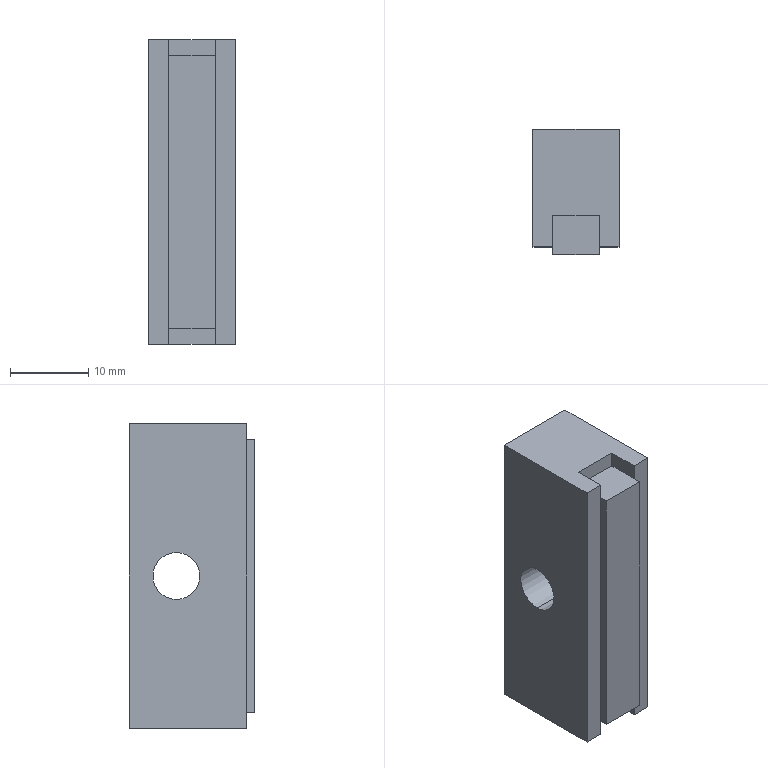Part | SolidWorks | features ICE 2, Extrusion 1 | 2 solids | 18 faces | box 11 x 16 x 39 mm | volume 6238 mm3 | plane 16 | cylinder 2 | commonest cylinder face diameters 6 x2
STEP:
#1=CARTESIAN_POINT('',(3.,-3.5,-17.5));
#2=VERTEX_POINT('',#1);
#3=CARTESIAN_POINT('',(3.,-3.5,17.5));
#4=VERTEX_POINT('',#3);
#5=CARTESIAN_POINT('',(3.,-3.5,-17.5));
#6=DIRECTION('',(0.,0.,1.));
#7=VECTOR('',#6,1000.);
#8=LINE('',#5,#7);
#9=EDGE_CURVE('',#2,#4,#8,.T.);
#10=ORIENTED_EDGE('',*,*,#9,.T.);
#11=CARTESIAN_POINT('',(3.,-8.5,17.5));
#12=VERTEX_POINT('',#11);
#13=CARTESIAN_POINT('',(3.,-8.5,17.5));
#14=DIRECTION('',(0.,1.,0.));
#15=VECTOR('',#14,1000.);
#16=LINE('',#13,#15);
#17=EDGE_CURVE('',#12,#4,#16,.T.);
#18=ORIENTED_EDGE('',*,*,#17,.F.);
#19=CARTESIAN_POINT('',(3.,-8.5,-17.5));
#20=VERTEX_POINT('',#19);
#21=CARTESIAN_POINT('',(3.,-8.5,-17.5));
#22=DIRECTION('',(0.,0.,1.));
#23=VECTOR('',#22,1000.);
#24=LINE('',#21,#23);
#25=EDGE_CURVE('',#20,#12,#24,.T.);
#26=ORIENTED_EDGE('',*,*,#25,.F.);
#27=CARTESIAN_POINT('',(3.,-8.5,-17.5));
#28=DIRECTION('',(0.,1.,0.));
#29=VECTOR('',#28,1000.);
#30=LINE('',#27,#29);
#31=EDGE_CURVE('',#20,#2,#30,.T.);
#32=ORIENTED_EDGE('',*,*,#31,.T.);
#33=EDGE_LOOP('',(#10,#18,#26,#32));
#34=FACE_OUTER_BOUND('',#33,.T.);
#35=CARTESIAN_POINT('',(3.,-8.5,-17.5));
#36=DIRECTION('',(-1.,0.,0.));
#37=DIRECTION('',(0.,0.,1.));
#38=AXIS2_PLACEMENT_3D('',#35,#36,#37);
#39=PLANE('',#38);
#40=ADVANCED_FACE('',(#34),#39,.F.);
#41=CARTESIAN_POINT('',(-3.,-3.5,17.5));
#42=VERTEX_POINT('',#41);
#43=CARTESIAN_POINT('',(-3.,-3.5,17.5));
#44=DIRECTION('',(-1.,0.,0.));
#45=VECTOR('',#44,1000.);
#46=LINE('',#43,#45);
#47=EDGE_CURVE('',#4,#42,#46,.T.);
#48=ORIENTED_EDGE('',*,*,#47,.T.);
#49=CARTESIAN_POINT('',(-3.,-8.5,17.5));
#50=VERTEX_POINT('',#49);
#51=CARTESIAN_POINT('',(-3.,-8.5,17.5));
#52=DIRECTION('',(0.,1.,0.));
#53=VECTOR('',#52,1000.);
#54=LINE('',#51,#53);
#55=EDGE_CURVE('',#50,#42,#54,.T.);
#56=ORIENTED_EDGE('',*,*,#55,.F.);
#57=CARTESIAN_POINT('',(-3.,-8.5,17.5));
#58=DIRECTION('',(-1.,0.,0.));
#59=VECTOR('',#58,1000.);
#60=LINE('',#57,#59);
#61=EDGE_CURVE('',#12,#50,#60,.T.);
#62=ORIENTED_EDGE('',*,*,#61,.F.);
#63=ORIENTED_EDGE('',*,*,#17,.T.);
#64=EDGE_LOOP('',(#48,#56,#62,#63));
#65=FACE_OUTER_BOUND('',#64,.T.);
#66=CARTESIAN_POINT('',(-3.,-8.5,17.5));
#67=DIRECTION('',(0.,0.,-1.));
#68=DIRECTION('',(-1.,0.,0.));
#69=AXIS2_PLACEMENT_3D('',#66,#67,#68);
#70=PLANE('',#69);
#71=ADVANCED_FACE('',(#65),#70,.F.);
#72=CARTESIAN_POINT('',(-3.,-3.5,-17.5));
#73=VERTEX_POINT('',#72);
#74=CARTESIAN_POINT('',(-3.,-3.5,-17.5));
#75=DIRECTION('',(0.,0.,-1.));
#76=VECTOR('',#75,1000.);
#77=LINE('',#74,#76);
#78=EDGE_CURVE('',#42,#73,#77,.T.);
#79=ORIENTED_EDGE('',*,*,#78,.T.);
#80=CARTESIAN_POINT('',(-3.,-8.5,-17.5));
#81=VERTEX_POINT('',#80);
#82=CARTESIAN_POINT('',(-3.,-8.5,-17.5));
#83=DIRECTION('',(0.,1.,0.));
#84=VECTOR('',#83,1000.);
#85=LINE('',#82,#84);
#86=EDGE_CURVE('',#81,#73,#85,.T.);
#87=ORIENTED_EDGE('',*,*,#86,.F.);
#88=CARTESIAN_POINT('',(-3.,-8.5,-17.5));
#89=DIRECTION('',(0.,0.,-1.));
#90=VECTOR('',#89,1000.);
#91=LINE('',#88,#90);
#92=EDGE_CURVE('',#50,#81,#91,.T.);
#93=ORIENTED_EDGE('',*,*,#92,.F.);
#94=ORIENTED_EDGE('',*,*,#55,.T.);
#95=EDGE_LOOP('',(#79,#87,#93,#94));
#96=FACE_OUTER_BOUND('',#95,.T.);
#97=CARTESIAN_POINT('',(-3.,-8.5,-17.5));
#98=DIRECTION('',(1.,0.,0.));
#99=DIRECTION('',(0.,0.,-1.));
#100=AXIS2_PLACEMENT_3D('',#97,#98,#99);
#101=PLANE('',#100);
#102=ADVANCED_FACE('',(#96),#101,.F.);
#103=CARTESIAN_POINT('',(-3.,-3.5,-17.5));
#104=DIRECTION('',(1.,0.,0.));
#105=VECTOR('',#104,1000.);
#106=LINE('',#103,#105);
#107=EDGE_CURVE('',#73,#2,#106,.T.);
#108=ORIENTED_EDGE('',*,*,#107,.T.);
#109=ORIENTED_EDGE('',*,*,#31,.F.);
#110=CARTESIAN_POINT('',(-3.,-8.5,-17.5));
#111=DIRECTION('',(1.,0.,0.));
#112=VECTOR('',#111,1000.);
#113=LINE('',#110,#112);
#114=EDGE_CURVE('',#81,#20,#113,.T.);
#115=ORIENTED_EDGE('',*,*,#114,.F.);
#116=ORIENTED_EDGE('',*,*,#86,.T.);
#117=EDGE_LOOP('',(#108,#109,#115,#116));
#118=FACE_OUTER_BOUND('',#117,.T.);
#119=CARTESIAN_POINT('',(-3.,-8.5,-17.5));
#120=DIRECTION('',(0.,0.,1.));
#121=DIRECTION('',(1.,0.,0.));
#122=AXIS2_PLACEMENT_3D('',#119,#120,#121);
#123=PLANE('',#122);
#124=ADVANCED_FACE('',(#118),#123,.F.);
#125=ORIENTED_EDGE('',*,*,#25,.T.);
#126=ORIENTED_EDGE('',*,*,#61,.T.);
#127=ORIENTED_EDGE('',*,*,#92,.T.);
#128=ORIENTED_EDGE('',*,*,#114,.T.);
#129=EDGE_LOOP('',(#125,#126,#127,#128));
#130=FACE_OUTER_BOUND('',#129,.T.);
#131=CARTESIAN_POINT('',(0.,-8.5,0.));
#132=DIRECTION('',(0.,1.,0.));
#133=DIRECTION('',(0.,0.,1.));
#134=AXIS2_PLACEMENT_3D('',#131,#132,#133);
#135=PLANE('',#134);
#136=ADVANCED_FACE('',(#130),#135,.F.);
#137=ORIENTED_EDGE('',*,*,#9,.F.);
#138=ORIENTED_EDGE('',*,*,#107,.F.);
#139=ORIENTED_EDGE('',*,*,#78,.F.);
#140=ORIENTED_EDGE('',*,*,#47,.F.);
#141=EDGE_LOOP('',(#137,#138,#139,#140));
#142=FACE_OUTER_BOUND('',#141,.T.);
#143=CARTESIAN_POINT('',(0.,-3.5,0.));
#144=DIRECTION('',(0.,1.,0.));
#145=DIRECTION('',(0.,0.,1.));
#146=AXIS2_PLACEMENT_3D('',#143,#144,#145);
#147=PLANE('',#146);
#148=ADVANCED_FACE('',(#142),#147,.T.);
#149=CLOSED_SHELL('',(#40,#71,#102,#124,#136,#148));
#150=MANIFOLD_SOLID_BREP('',#149);
#151=CARTESIAN_POINT('',(5.5,1.5,3.));
#152=VERTEX_POINT('',#151);
#153=CARTESIAN_POINT('',(5.5,1.5,-3.));
#154=VERTEX_POINT('',#153);
#155=CARTESIAN_POINT('',(5.5,1.5,0.));
#156=DIRECTION('',(1.,0.,0.));
#157=DIRECTION('',(0.,0.,1.));
#158=AXIS2_PLACEMENT_3D('',#155,#156,#157);
#159=CIRCLE('',#158,3.);
#160=EDGE_CURVE('',#152,#154,#159,.T.);
#161=ORIENTED_EDGE('',*,*,#160,.T.);
#162=CARTESIAN_POINT('',(-5.5,1.5,-3.));
#163=VERTEX_POINT('',#162);
#164=CARTESIAN_POINT('',(5.501,1.5,-3.));
#165=DIRECTION('',(-1.,0.,0.));
#166=VECTOR('',#165,1000.);
#167=LINE('',#164,#166);
#168=EDGE_CURVE('',#154,#163,#167,.T.);
#169=ORIENTED_EDGE('',*,*,#168,.T.);
#170=CARTESIAN_POINT('',(-5.5,1.5,3.));
#171=VERTEX_POINT('',#170);
#172=CARTESIAN_POINT('',(-5.5,1.5,0.));
#173=DIRECTION('',(-1.,0.,0.));
#174=DIRECTION('',(0.,0.,1.));
#175=AXIS2_PLACEMENT_3D('',#172,#173,#174);
#176=CIRCLE('',#175,3.);
#177=EDGE_CURVE('',#163,#171,#176,.T.);
#178=ORIENTED_EDGE('',*,*,#177,.T.);
#179=CARTESIAN_POINT('',(5.501,1.5,3.));
#180=DIRECTION('',(-1.,0.,0.));
#181=VECTOR('',#180,1000.);
#182=LINE('',#179,#181);
#183=EDGE_CURVE('',#152,#171,#182,.T.);
#184=ORIENTED_EDGE('',*,*,#183,.F.);
#185=EDGE_LOOP('',(#161,#169,#178,#184));
#186=FACE_OUTER_BOUND('',#185,.T.);
#187=CARTESIAN_POINT('',(5.501,1.5,0.));
#188=DIRECTION('',(-1.,0.,0.));
#189=DIRECTION('',(0.,0.,1.));
#190=AXIS2_PLACEMENT_3D('',#187,#188,#189);
#191=CYLINDRICAL_SURFACE('',#190,3.);
#192=ADVANCED_FACE('',(#186),#191,.F.);
#193=ORIENTED_EDGE('',*,*,#160,.F.);
#194=CARTESIAN_POINT('',(5.5,1.5,0.));
#195=DIRECTION('',(1.,0.,0.));
#196=DIRECTION('',(0.,0.,1.));
#197=AXIS2_PLACEMENT_3D('',#194,#195,#196);
#198=CIRCLE('',#197,3.);
#199=EDGE_CURVE('',#154,#152,#198,.T.);
#200=ORIENTED_EDGE('',*,*,#199,.F.);
#201=EDGE_LOOP('',(#193,#200));
#202=FACE_BOUND('',#201,.T.);
#203=CARTESIAN_POINT('',(5.5,-7.5,-19.5));
#204=VERTEX_POINT('',#203);
#205=CARTESIAN_POINT('',(5.5,7.5,-19.5));
#206=VERTEX_POINT('',#205);
#207=CARTESIAN_POINT('',(5.5,-7.5,-19.5));
#208=DIRECTION('',(0.,1.,0.));
#209=VECTOR('',#208,1000.);
#210=LINE('',#207,#209);
#211=EDGE_CURVE('',#204,#206,#210,.T.);
#212=ORIENTED_EDGE('',*,*,#211,.T.);
#213=CARTESIAN_POINT('',(5.5,7.5,19.5));
#214=VERTEX_POINT('',#213);
#215=CARTESIAN_POINT('',(5.5,7.5,19.5));
#216=DIRECTION('',(0.,0.,-1.));
#217=VECTOR('',#216,1000.);
#218=LINE('',#215,#217);
#219=EDGE_CURVE('',#214,#206,#218,.T.);
#220=ORIENTED_EDGE('',*,*,#219,.F.);
#221=CARTESIAN_POINT('',(5.5,-7.5,19.5));
#222=VERTEX_POINT('',#221);
#223=CARTESIAN_POINT('',(5.5,-7.5,19.5));
#224=DIRECTION('',(0.,1.,0.));
#225=VECTOR('',#224,1000.);
#226=LINE('',#223,#225);
#227=EDGE_CURVE('',#222,#214,#226,.T.);
#228=ORIENTED_EDGE('',*,*,#227,.F.);
#229=CARTESIAN_POINT('',(5.5,-7.5,19.5));
#230=DIRECTION('',(0.,0.,-1.));
#231=VECTOR('',#230,1000.);
#232=LINE('',#229,#231);
#233=EDGE_CURVE('',#222,#204,#232,.T.);
#234=ORIENTED_EDGE('',*,*,#233,.T.);
#235=EDGE_LOOP('',(#212,#220,#228,#234));
#236=FACE_OUTER_BOUND('',#235,.T.);
#237=CARTESIAN_POINT('',(5.5,-7.5,19.5));
#238=DIRECTION('',(-1.,0.,0.));
#239=DIRECTION('',(0.,0.,1.));
#240=AXIS2_PLACEMENT_3D('',#237,#238,#239);
#241=PLANE('',#240);
#242=ADVANCED_FACE('',(#202,#236),#241,.F.);
#243=CARTESIAN_POINT('',(-5.5,7.5,-19.5));
#244=VERTEX_POINT('',#243);
#245=CARTESIAN_POINT('',(-5.5,7.5,-19.5));
#246=DIRECTION('',(-1.,0.,0.));
#247=VECTOR('',#246,1000.);
#248=LINE('',#245,#247);
#249=EDGE_CURVE('',#206,#244,#248,.T.);
#250=ORIENTED_EDGE('',*,*,#249,.T.);
#251=CARTESIAN_POINT('',(-5.5,7.5,19.5));
#252=VERTEX_POINT('',#251);
#253=CARTESIAN_POINT('',(-5.5,7.5,19.5));
#254=DIRECTION('',(0.,0.,-1.));
#255=VECTOR('',#254,1000.);
#256=LINE('',#253,#255);
#257=EDGE_CURVE('',#252,#244,#256,.T.);
#258=ORIENTED_EDGE('',*,*,#257,.F.);
#259=CARTESIAN_POINT('',(-5.5,7.5,19.5));
#260=DIRECTION('',(-1.,0.,0.));
#261=VECTOR('',#260,1000.);
#262=LINE('',#259,#261);
#263=EDGE_CURVE('',#214,#252,#262,.T.);
#264=ORIENTED_EDGE('',*,*,#263,.F.);
#265=ORIENTED_EDGE('',*,*,#219,.T.);
#266=EDGE_LOOP('',(#250,#258,#264,#265));
#267=FACE_OUTER_BOUND('',#266,.T.);
#268=CARTESIAN_POINT('',(-5.5,7.5,19.5));
#269=DIRECTION('',(0.,-1.,0.));
#270=DIRECTION('',(0.,0.,-1.));
#271=AXIS2_PLACEMENT_3D('',#268,#269,#270);
#272=PLANE('',#271);
#273=ADVANCED_FACE('',(#267),#272,.F.);
#274=CARTESIAN_POINT('',(-5.5,1.5,0.));
#275=DIRECTION('',(-1.,0.,0.));
#276=DIRECTION('',(0.,0.,1.));
#277=AXIS2_PLACEMENT_3D('',#274,#275,#276);
#278=CIRCLE('',#277,3.);
#279=EDGE_CURVE('',#171,#163,#278,.T.);
#280=ORIENTED_EDGE('',*,*,#279,.F.);
#281=ORIENTED_EDGE('',*,*,#177,.F.);
#282=EDGE_LOOP('',(#280,#281));
#283=FACE_BOUND('',#282,.T.);
#284=CARTESIAN_POINT('',(-5.5,-7.5,-19.5));
#285=VERTEX_POINT('',#284);
#286=CARTESIAN_POINT('',(-5.5,-7.5,-19.5));
#287=DIRECTION('',(0.,-1.,0.));
#288=VECTOR('',#287,1000.);
#289=LINE('',#286,#288);
#290=EDGE_CURVE('',#244,#285,#289,.T.);
#291=ORIENTED_EDGE('',*,*,#290,.T.);
#292=CARTESIAN_POINT('',(-5.5,-7.5,19.5));
#293=VERTEX_POINT('',#292);
#294=CARTESIAN_POINT('',(-5.5,-7.5,19.5));
#295=DIRECTION('',(0.,0.,-1.));
#296=VECTOR('',#295,1000.);
#297=LINE('',#294,#296);
#298=EDGE_CURVE('',#293,#285,#297,.T.);
#299=ORIENTED_EDGE('',*,*,#298,.F.);
#300=CARTESIAN_POINT('',(-5.5,-7.5,19.5));
#301=DIRECTION('',(0.,-1.,0.));
#302=VECTOR('',#301,1000.);
#303=LINE('',#300,#302);
#304=EDGE_CURVE('',#252,#293,#303,.T.);
#305=ORIENTED_EDGE('',*,*,#304,.F.);
#306=ORIENTED_EDGE('',*,*,#257,.T.);
#307=EDGE_LOOP('',(#291,#299,#305,#306));
#308=FACE_OUTER_BOUND('',#307,.T.);
#309=CARTESIAN_POINT('',(-5.5,-7.5,19.5));
#310=DIRECTION('',(1.,0.,0.));
#311=DIRECTION('',(0.,0.,-1.));
#312=AXIS2_PLACEMENT_3D('',#309,#310,#311);
#313=PLANE('',#312);
#314=ADVANCED_FACE('',(#283,#308),#313,.F.);
#315=CARTESIAN_POINT('',(-3.,-7.5,-19.5));
#316=VERTEX_POINT('',#315);
#317=CARTESIAN_POINT('',(-5.5,-7.5,-19.5));
#318=DIRECTION('',(1.,0.,0.));
#319=VECTOR('',#318,1000.);
#320=LINE('',#317,#319);
#321=EDGE_CURVE('',#285,#316,#320,.T.);
#322=ORIENTED_EDGE('',*,*,#321,.T.);
#323=CARTESIAN_POINT('',(-3.,-7.5,19.5));
#324=VERTEX_POINT('',#323);
#325=CARTESIAN_POINT('',(-3.,-7.5,19.5));
#326=DIRECTION('',(0.,0.,-1.));
#327=VECTOR('',#326,1000.);
#328=LINE('',#325,#327);
#329=EDGE_CURVE('',#324,#316,#328,.T.);
#330=ORIENTED_EDGE('',*,*,#329,.F.);
#331=CARTESIAN_POINT('',(-5.5,-7.5,19.5));
#332=DIRECTION('',(1.,0.,0.));
#333=VECTOR('',#332,1000.);
#334=LINE('',#331,#333);
#335=EDGE_CURVE('',#293,#324,#334,.T.);
#336=ORIENTED_EDGE('',*,*,#335,.F.);
#337=ORIENTED_EDGE('',*,*,#298,.T.);
#338=EDGE_LOOP('',(#322,#330,#336,#337));
#339=FACE_OUTER_BOUND('',#338,.T.);
#340=CARTESIAN_POINT('',(-5.5,-7.5,19.5));
#341=DIRECTION('',(0.,1.,0.));
#342=DIRECTION('',(0.,0.,1.));
#343=AXIS2_PLACEMENT_3D('',#340,#341,#342);
#344=PLANE('',#343);
#345=ADVANCED_FACE('',(#339),#344,.F.);
#346=CARTESIAN_POINT('',(-3.,-3.5,-19.5));
#347=VERTEX_POINT('',#346);
#348=CARTESIAN_POINT('',(-3.,-7.5,-19.5));
#349=DIRECTION('',(0.,1.,0.));
#350=VECTOR('',#349,1000.);
#351=LINE('',#348,#350);
#352=EDGE_CURVE('',#316,#347,#351,.T.);
#353=ORIENTED_EDGE('',*,*,#352,.T.);
#354=CARTESIAN_POINT('',(-3.,-3.5,19.5));
#355=VERTEX_POINT('',#354);
#356=CARTESIAN_POINT('',(-3.,-3.5,19.5));
#357=DIRECTION('',(0.,0.,-1.));
#358=VECTOR('',#357,1000.);
#359=LINE('',#356,#358);
#360=EDGE_CURVE('',#355,#347,#359,.T.);
#361=ORIENTED_EDGE('',*,*,#360,.F.);
#362=CARTESIAN_POINT('',(-3.,-7.5,19.5));
#363=DIRECTION('',(0.,1.,0.));
#364=VECTOR('',#363,1000.);
#365=LINE('',#362,#364);
#366=EDGE_CURVE('',#324,#355,#365,.T.);
#367=ORIENTED_EDGE('',*,*,#366,.F.);
#368=ORIENTED_EDGE('',*,*,#329,.T.);
#369=EDGE_LOOP('',(#353,#361,#367,#368));
#370=FACE_OUTER_BOUND('',#369,.T.);
#371=CARTESIAN_POINT('',(-3.,-7.5,19.5));
#372=DIRECTION('',(-1.,0.,0.));
#373=DIRECTION('',(0.,0.,1.));
#374=AXIS2_PLACEMENT_3D('',#371,#372,#373);
#375=PLANE('',#374);
#376=ADVANCED_FACE('',(#370),#375,.F.);
#377=CARTESIAN_POINT('',(3.,-3.5,-19.5));
#378=VERTEX_POINT('',#377);
#379=CARTESIAN_POINT('',(-3.,-3.5,-19.5));
#380=DIRECTION('',(1.,0.,0.));
#381=VECTOR('',#380,1000.);
#382=LINE('',#379,#381);
#383=EDGE_CURVE('',#347,#378,#382,.T.);
#384=ORIENTED_EDGE('',*,*,#383,.T.);
#385=CARTESIAN_POINT('',(3.,-3.5,19.5));
#386=VERTEX_POINT('',#385);
#387=CARTESIAN_POINT('',(3.,-3.5,19.5));
#388=DIRECTION('',(0.,0.,-1.));
#389=VECTOR('',#388,1000.);
#390=LINE('',#387,#389);
#391=EDGE_CURVE('',#386,#378,#390,.T.);
#392=ORIENTED_EDGE('',*,*,#391,.F.);
#393=CARTESIAN_POINT('',(-3.,-3.5,19.5));
#394=DIRECTION('',(1.,0.,0.));
#395=VECTOR('',#394,1000.);
#396=LINE('',#393,#395);
#397=EDGE_CURVE('',#355,#386,#396,.T.);
#398=ORIENTED_EDGE('',*,*,#397,.F.);
#399=ORIENTED_EDGE('',*,*,#360,.T.);
#400=EDGE_LOOP('',(#384,#392,#398,#399));
#401=FACE_OUTER_BOUND('',#400,.T.);
#402=CARTESIAN_POINT('',(-3.,-3.5,19.5));
#403=DIRECTION('',(0.,1.,0.));
#404=DIRECTION('',(0.,0.,1.));
#405=AXIS2_PLACEMENT_3D('',#402,#403,#404);
#406=PLANE('',#405);
#407=ADVANCED_FACE('',(#401),#406,.F.);
#408=CARTESIAN_POINT('',(3.,-7.5,-19.5));
#409=VERTEX_POINT('',#408);
#410=CARTESIAN_POINT('',(3.,-7.5,-19.5));
#411=DIRECTION('',(0.,-1.,0.));
#412=VECTOR('',#411,1000.);
#413=LINE('',#410,#412);
#414=EDGE_CURVE('',#378,#409,#413,.T.);
#415=ORIENTED_EDGE('',*,*,#414,.T.);
#416=CARTESIAN_POINT('',(3.,-7.5,19.5));
#417=VERTEX_POINT('',#416);
#418=CARTESIAN_POINT('',(3.,-7.5,19.5));
#419=DIRECTION('',(0.,0.,-1.));
#420=VECTOR('',#419,1000.);
#421=LINE('',#418,#420);
#422=EDGE_CURVE('',#417,#409,#421,.T.);
#423=ORIENTED_EDGE('',*,*,#422,.F.);
#424=CARTESIAN_POINT('',(3.,-7.5,19.5));
#425=DIRECTION('',(0.,-1.,0.));
#426=VECTOR('',#425,1000.);
#427=LINE('',#424,#426);
#428=EDGE_CURVE('',#386,#417,#427,.T.);
#429=ORIENTED_EDGE('',*,*,#428,.F.);
#430=ORIENTED_EDGE('',*,*,#391,.T.);
#431=EDGE_LOOP('',(#415,#423,#429,#430));
#432=FACE_OUTER_BOUND('',#431,.T.);
#433=CARTESIAN_POINT('',(3.,-7.5,19.5));
#434=DIRECTION('',(1.,0.,0.));
#435=DIRECTION('',(0.,0.,-1.));
#436=AXIS2_PLACEMENT_3D('',#433,#434,#435);
#437=PLANE('',#436);
#438=ADVANCED_FACE('',(#432),#437,.F.);
#439=CARTESIAN_POINT('',(3.,-7.5,-19.5));
#440=DIRECTION('',(1.,0.,0.));
#441=VECTOR('',#440,1000.);
#442=LINE('',#439,#441);
#443=EDGE_CURVE('',#409,#204,#442,.T.);
#444=ORIENTED_EDGE('',*,*,#443,.T.);
#445=ORIENTED_EDGE('',*,*,#233,.F.);
#446=CARTESIAN_POINT('',(3.,-7.5,19.5));
#447=DIRECTION('',(1.,0.,0.));
#448=VECTOR('',#447,1000.);
#449=LINE('',#446,#448);
#450=EDGE_CURVE('',#417,#222,#449,.T.);
#451=ORIENTED_EDGE('',*,*,#450,.F.);
#452=ORIENTED_EDGE('',*,*,#422,.T.);
#453=EDGE_LOOP('',(#444,#445,#451,#452));
#454=FACE_OUTER_BOUND('',#453,.T.);
#455=CARTESIAN_POINT('',(3.,-7.5,19.5));
#456=DIRECTION('',(0.,1.,0.));
#457=DIRECTION('',(0.,0.,1.));
#458=AXIS2_PLACEMENT_3D('',#455,#456,#457);
#459=PLANE('',#458);
#460=ADVANCED_FACE('',(#454),#459,.F.);
#461=ORIENTED_EDGE('',*,*,#227,.T.);
#462=ORIENTED_EDGE('',*,*,#263,.T.);
#463=ORIENTED_EDGE('',*,*,#304,.T.);
#464=ORIENTED_EDGE('',*,*,#335,.T.);
#465=ORIENTED_EDGE('',*,*,#366,.T.);
#466=ORIENTED_EDGE('',*,*,#397,.T.);
#467=ORIENTED_EDGE('',*,*,#428,.T.);
#468=ORIENTED_EDGE('',*,*,#450,.T.);
#469=EDGE_LOOP('',(#461,#462,#463,#464,#465,#466,#467,#468));
#470=FACE_OUTER_BOUND('',#469,.T.);
#471=CARTESIAN_POINT('',(0.,0.,19.5));
#472=DIRECTION('',(0.,0.,-1.));
#473=DIRECTION('',(-1.,0.,0.));
#474=AXIS2_PLACEMENT_3D('',#471,#472,#473);
#475=PLANE('',#474);
#476=ADVANCED_FACE('',(#470),#475,.F.);
#477=ORIENTED_EDGE('',*,*,#211,.F.);
#478=ORIENTED_EDGE('',*,*,#443,.F.);
#479=ORIENTED_EDGE('',*,*,#414,.F.);
#480=ORIENTED_EDGE('',*,*,#383,.F.);
#481=ORIENTED_EDGE('',*,*,#352,.F.);
#482=ORIENTED_EDGE('',*,*,#321,.F.);
#483=ORIENTED_EDGE('',*,*,#290,.F.);
#484=ORIENTED_EDGE('',*,*,#249,.F.);
#485=EDGE_LOOP('',(#477,#478,#479,#480,#481,#482,#483,#484));
#486=FACE_OUTER_BOUND('',#485,.T.);
#487=CARTESIAN_POINT('',(0.,0.,-19.5));
#488=DIRECTION('',(0.,0.,-1.));
#489=DIRECTION('',(-1.,0.,0.));
#490=AXIS2_PLACEMENT_3D('',#487,#488,#489);
#491=PLANE('',#490);
#492=ADVANCED_FACE('',(#486),#491,.T.);
#493=ORIENTED_EDGE('',*,*,#168,.F.);
#494=ORIENTED_EDGE('',*,*,#199,.T.);
#495=ORIENTED_EDGE('',*,*,#183,.T.);
#496=ORIENTED_EDGE('',*,*,#279,.T.);
#497=EDGE_LOOP('',(#493,#494,#495,#496));
#498=FACE_OUTER_BOUND('',#497,.T.);
#499=CARTESIAN_POINT('',(5.501,1.5,0.));
#500=DIRECTION('',(-1.,0.,0.));
#501=DIRECTION('',(0.,0.,1.));
#502=AXIS2_PLACEMENT_3D('',#499,#500,#501);
#503=CYLINDRICAL_SURFACE('',#502,3.);
#504=ADVANCED_FACE('',(#498),#503,.F.);
#505=CLOSED_SHELL('',(#192,#242,#273,#314,#345,#376,#407,#438,#460,#476,#492,#504));
#506=MANIFOLD_SOLID_BREP('',#505);
#507=CARTESIAN_POINT('',(0.,0.,0.));
#508=DIRECTION('',(0.,0.,1.));
#509=DIRECTION('',(1.,0.,0.));
#510=AXIS2_PLACEMENT_3D('',#507,#508,#509);
#511=(LENGTH_UNIT()NAMED_UNIT(*)SI_UNIT(.MILLI.,.METRE.));
#512=UNCERTAINTY_MEASURE_WITH_UNIT(LENGTH_MEASURE(0.00001),#511,'','');
#513=(NAMED_UNIT(*)PLANE_ANGLE_UNIT()SI_UNIT($,.RADIAN.));
#514=(NAMED_UNIT(*)SI_UNIT($,.STERADIAN.)SOLID_ANGLE_UNIT());
#515=(GEOMETRIC_REPRESENTATION_CONTEXT(3)GLOBAL_UNCERTAINTY_ASSIGNED_CONTEXT((#512))GLOBAL_UNIT_ASSIGNED_CONTEXT((#511,#513,#514))REPRESENTATION_CONTEXT('',''));
#516=ADVANCED_BREP_SHAPE_REPRESENTATION('',(#150,#506,#510),#515);